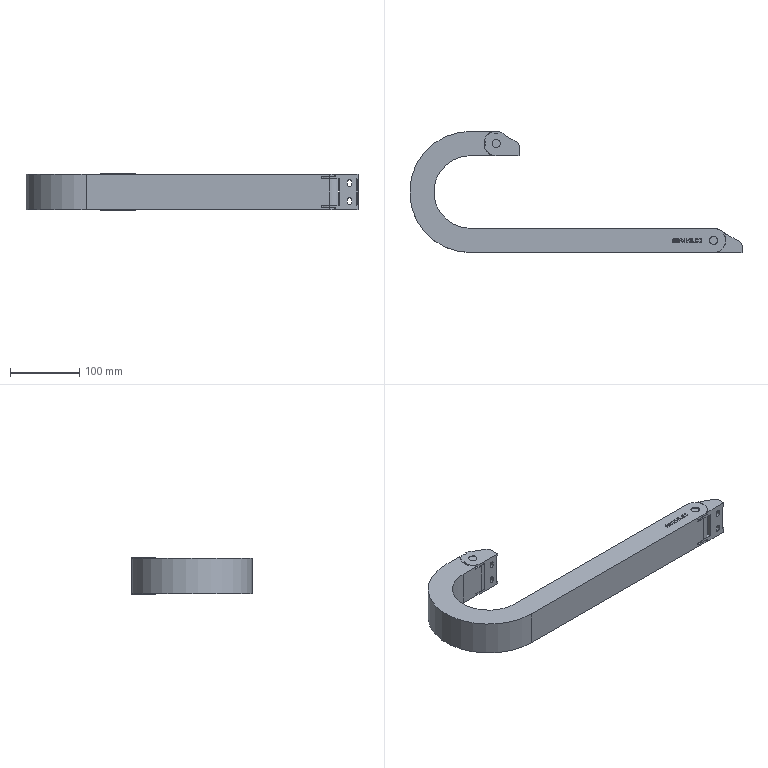Part | SolidWorks | features BaseBody 3 | 3 solids | 233 faces | box 480.2 x 175 x 53 mm | volume 549939 mm3 | plane 136 | cylinder 89 | spline 8 | commonest cylinder face diameters 35 x24 12 x16 4 x12 6.2 x12 1.407 x4 2.982 x4